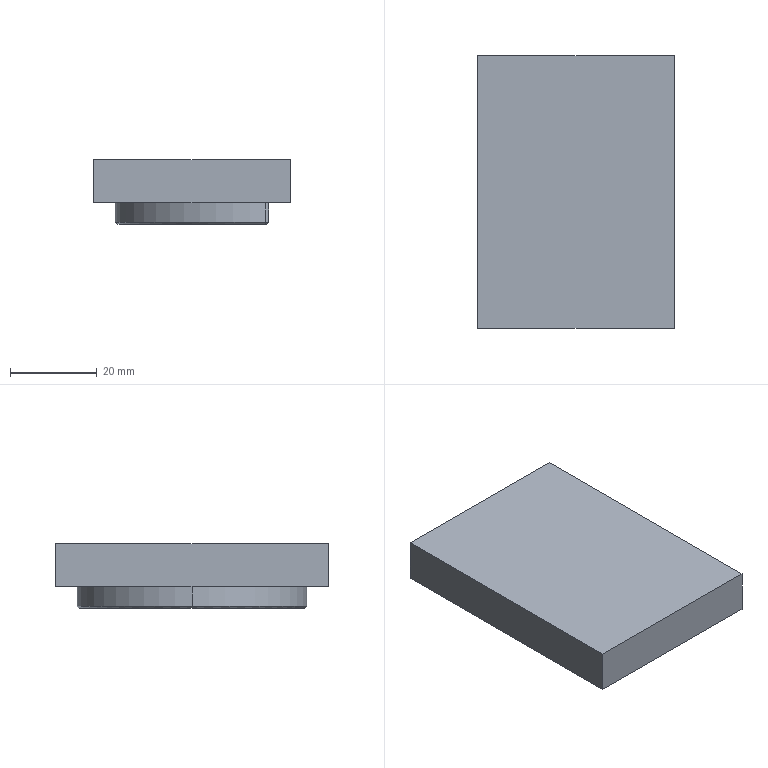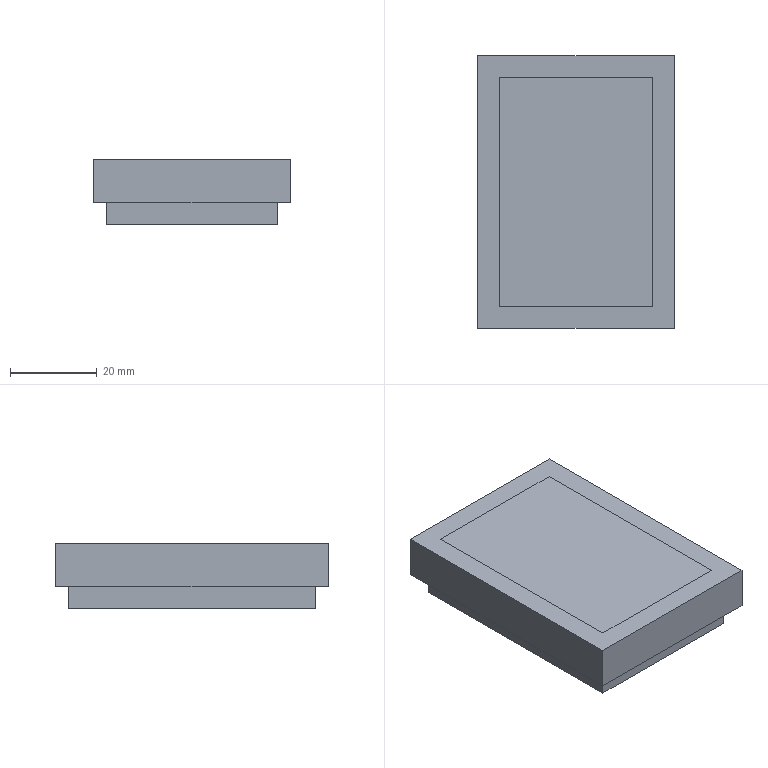CAM job | NX | 3-axis milling, drilling | part box 45.394 x 63 x 15 mm | stock box 45.394 x 63 x 15 mm
Tools:
number,name,description,diameter,corner_radius,flute_length,length,flutes
19,D80,Milling Tool-5 Parameters,80.0,0.0,50.0,75.0,2
14,D10JING,Milling Tool-5 Parameters,10.0,0.0,50.0,75.0,2
15,D10,Milling Tool-5 Parameters,10.0,0.0,50.0,75.0,2
1,D6A45,Milling Tool-5 Parameters,6.0,0.0,50.0,75.0,2
7,3.5ZT,Drilling Tool,3.4,0.0,35.0,50.0,2
11,D4,Milling Tool-5 Parameters,4.0,0.0,50.0,75.0,2
17,D2,Milling Tool-5 Parameters,2.0,0.0,50.0,75.0,2
Operations:
program,operation,operation_type,tool,method,geometry_group,spindle_rpm,surface_speed,feed_per_tooth,feed_cut,feed_plunge,cut_length_mm,path_length_mm,cut_time_min,machine_time_min
1,FLOOR_WALL,VolumeBased25DMillingOperation,D80,METHOD,A,5000.0,1256.0,0.12,1200.0,100.0,149.0,203.0,0.1242,0.1296
1,CAVITY_MILL,CavityMilling,D10,METHOD,A,9500.0,298.0,0.1842,3500.0,1000.0,3366.33,3537.235,1.019,1.036
1,ZLEVEL_PROFILE_COPY,ZLevelMilling,D10JING,METHOD,A,9500.0,298.0,0.0789,1500.0,1000.0,244.3,321.3,0.1724,0.1801
1,SPOT_DRILLING,Operation,D6A45,METHOD,A,9500.0,179.0,0.0132,250.0,0.0,16.0,166.464,0.064,0.079
1,DRILLING_COPY_COPY,Operation,3.5ZT,METHOD,A,2500.0,35.0,0.04,200.0,0.0,62.086,258.635,0.3104,0.3301
1,HOLE_MILLING_2,CylinderMilling,D4,METHOD,A,9500.0,119.0,0.0658,1250.0,100.0,283.239,609.166,0.2266,0.2592
1,PLANAR_PROFILE,PlanarMilling,D6A45,METHOD,A,9500.0,179.0,0.0789,1500.0,100.0,266.122,662.665,0.1774,0.2171
2,FLOOR_WALL_COPY,VolumeBased25DMillingOperation,D80,METHOD,B,5000.0,1256.0,0.12,1200.0,100.0,745.0,1567.001,0.6208,0.703
2,HOLE_MILLING_1,CylinderMilling,D2,METHOD,B,9500.0,59.0,0.0553,1050.0,100.0,121.233,185.733,0.1155,0.1219
2,PLANAR_PROFILE_1,PlanarMilling,D6A45,METHOD,B,9500.0,179.0,0.0789,1500.0,100.0,253.905,740.319,0.1693,0.2179
3工装,FLOOR_WALL_1_COPY_1,VolumeBased25DMillingOperation,D4,METHOD,C,9500.0,119.0,0.1053,2000.0,1000.0,4780.704,5959.432,2.624,2.742
3工装,FLOOR_WALL_1_COPY_1_COPY,VolumeBased25DMillingOperation,D4,METHOD,C,9500.0,119.0,0.1053,2000.0,1000.0,203.211,266.211,0.1094,0.1157